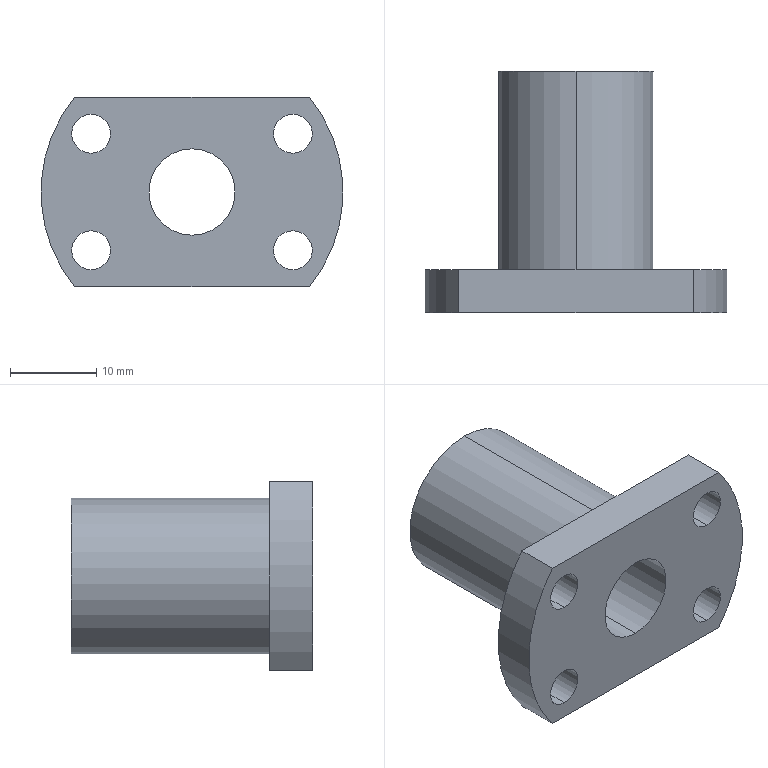Part | NX | features BREP 1 | 1 solid | 19 faces | box 35 x 28 x 22 mm | volume 6914 mm3 | cylinder 14 | plane 5 | commonest cylinder face diameters 4.5 x8 10 x2 18 x2 35 x2
STEP:
#1=CARTESIAN_POINT('',(-11.691,5.,-4.5));
#2=VERTEX_POINT('',#1);
#3=CARTESIAN_POINT('',(-11.691,0.,-4.5));
#4=VERTEX_POINT('',#3);
#5=CARTESIAN_POINT('',(-11.691,0.,-4.5));
#6=DIRECTION('',(0.,-1.,0.));
#7=VECTOR('',#6,1000.);
#8=LINE('',#5,#7);
#9=EDGE_CURVE('',#2,#4,#8,.T.);
#10=ORIENTED_EDGE('',*,*,#9,.F.);
#11=CARTESIAN_POINT('',(-11.691,5.,-9.));
#12=VERTEX_POINT('',#11);
#13=CARTESIAN_POINT('',(-11.691,5.,-6.75));
#14=DIRECTION('',(0.,-1.,0.));
#15=DIRECTION('',(0.,0.,-1.));
#16=AXIS2_PLACEMENT_3D('',#13,#14,#15);
#17=CIRCLE('',#16,2.25);
#18=EDGE_CURVE('',#12,#2,#17,.T.);
#19=ORIENTED_EDGE('',*,*,#18,.F.);
#20=CARTESIAN_POINT('',(-11.691,0.,-9.));
#21=VERTEX_POINT('',#20);
#22=CARTESIAN_POINT('',(-11.691,0.,-9.));
#23=DIRECTION('',(0.,-1.,0.));
#24=VECTOR('',#23,1000.);
#25=LINE('',#22,#24);
#26=EDGE_CURVE('',#12,#21,#25,.T.);
#27=ORIENTED_EDGE('',*,*,#26,.T.);
#28=CARTESIAN_POINT('',(-11.691,0.,-6.75));
#29=DIRECTION('',(0.,-1.,0.));
#30=DIRECTION('',(0.,0.,-1.));
#31=AXIS2_PLACEMENT_3D('',#28,#29,#30);
#32=CIRCLE('',#31,2.25);
#33=EDGE_CURVE('',#21,#4,#32,.T.);
#34=ORIENTED_EDGE('',*,*,#33,.T.);
#35=EDGE_LOOP('',(#10,#19,#27,#34));
#36=FACE_BOUND('',#35,.T.);
#37=CARTESIAN_POINT('',(-11.691,0.,-6.75));
#38=DIRECTION('',(0.,-1.,0.));
#39=DIRECTION('',(0.,0.,-1.));
#40=AXIS2_PLACEMENT_3D('',#37,#38,#39);
#41=CYLINDRICAL_SURFACE('',#40,2.25);
#42=ADVANCED_FACE('',(#36),#41,.F.);
#43=CARTESIAN_POINT('',(-11.691,5.,9.));
#44=VERTEX_POINT('',#43);
#45=CARTESIAN_POINT('',(-11.691,0.,9.));
#46=VERTEX_POINT('',#45);
#47=CARTESIAN_POINT('',(-11.691,0.,9.));
#48=DIRECTION('',(0.,-1.,0.));
#49=VECTOR('',#48,1000.);
#50=LINE('',#47,#49);
#51=EDGE_CURVE('',#44,#46,#50,.T.);
#52=ORIENTED_EDGE('',*,*,#51,.F.);
#53=CARTESIAN_POINT('',(-11.691,5.,4.5));
#54=VERTEX_POINT('',#53);
#55=CARTESIAN_POINT('',(-11.691,5.,6.75));
#56=DIRECTION('',(0.,-1.,0.));
#57=DIRECTION('',(0.,0.,-1.));
#58=AXIS2_PLACEMENT_3D('',#55,#56,#57);
#59=CIRCLE('',#58,2.25);
#60=EDGE_CURVE('',#54,#44,#59,.T.);
#61=ORIENTED_EDGE('',*,*,#60,.F.);
#62=CARTESIAN_POINT('',(-11.691,0.,4.5));
#63=VERTEX_POINT('',#62);
#64=CARTESIAN_POINT('',(-11.691,0.,4.5));
#65=DIRECTION('',(0.,-1.,0.));
#66=VECTOR('',#65,1000.);
#67=LINE('',#64,#66);
#68=EDGE_CURVE('',#54,#63,#67,.T.);
#69=ORIENTED_EDGE('',*,*,#68,.T.);
#70=CARTESIAN_POINT('',(-11.691,0.,6.75));
#71=DIRECTION('',(0.,-1.,0.));
#72=DIRECTION('',(0.,0.,-1.));
#73=AXIS2_PLACEMENT_3D('',#70,#71,#72);
#74=CIRCLE('',#73,2.25);
#75=EDGE_CURVE('',#63,#46,#74,.T.);
#76=ORIENTED_EDGE('',*,*,#75,.T.);
#77=EDGE_LOOP('',(#52,#61,#69,#76));
#78=FACE_BOUND('',#77,.T.);
#79=CARTESIAN_POINT('',(-11.691,0.,6.75));
#80=DIRECTION('',(0.,-1.,0.));
#81=DIRECTION('',(0.,0.,-1.));
#82=AXIS2_PLACEMENT_3D('',#79,#80,#81);
#83=CYLINDRICAL_SURFACE('',#82,2.25);
#84=ADVANCED_FACE('',(#78),#83,.F.);
#85=CARTESIAN_POINT('',(11.691,5.,-4.5));
#86=VERTEX_POINT('',#85);
#87=CARTESIAN_POINT('',(11.691,0.,-4.5));
#88=VERTEX_POINT('',#87);
#89=CARTESIAN_POINT('',(11.691,0.,-4.5));
#90=DIRECTION('',(0.,-1.,0.));
#91=VECTOR('',#90,1000.);
#92=LINE('',#89,#91);
#93=EDGE_CURVE('',#86,#88,#92,.T.);
#94=ORIENTED_EDGE('',*,*,#93,.F.);
#95=CARTESIAN_POINT('',(11.691,5.,-9.));
#96=VERTEX_POINT('',#95);
#97=CARTESIAN_POINT('',(11.691,5.,-6.75));
#98=DIRECTION('',(0.,-1.,0.));
#99=DIRECTION('',(0.,0.,-1.));
#100=AXIS2_PLACEMENT_3D('',#97,#98,#99);
#101=CIRCLE('',#100,2.25);
#102=EDGE_CURVE('',#96,#86,#101,.T.);
#103=ORIENTED_EDGE('',*,*,#102,.F.);
#104=CARTESIAN_POINT('',(11.691,0.,-9.));
#105=VERTEX_POINT('',#104);
#106=CARTESIAN_POINT('',(11.691,0.,-9.));
#107=DIRECTION('',(0.,-1.,0.));
#108=VECTOR('',#107,1000.);
#109=LINE('',#106,#108);
#110=EDGE_CURVE('',#96,#105,#109,.T.);
#111=ORIENTED_EDGE('',*,*,#110,.T.);
#112=CARTESIAN_POINT('',(11.691,0.,-6.75));
#113=DIRECTION('',(0.,-1.,0.));
#114=DIRECTION('',(0.,0.,-1.));
#115=AXIS2_PLACEMENT_3D('',#112,#113,#114);
#116=CIRCLE('',#115,2.25);
#117=EDGE_CURVE('',#105,#88,#116,.T.);
#118=ORIENTED_EDGE('',*,*,#117,.T.);
#119=EDGE_LOOP('',(#94,#103,#111,#118));
#120=FACE_BOUND('',#119,.T.);
#121=CARTESIAN_POINT('',(11.691,0.,-6.75));
#122=DIRECTION('',(0.,-1.,0.));
#123=DIRECTION('',(0.,0.,-1.));
#124=AXIS2_PLACEMENT_3D('',#121,#122,#123);
#125=CYLINDRICAL_SURFACE('',#124,2.25);
#126=ADVANCED_FACE('',(#120),#125,.F.);
#127=CARTESIAN_POINT('',(11.691,5.,9.));
#128=VERTEX_POINT('',#127);
#129=CARTESIAN_POINT('',(11.691,0.,9.));
#130=VERTEX_POINT('',#129);
#131=CARTESIAN_POINT('',(11.691,0.,9.));
#132=DIRECTION('',(0.,-1.,0.));
#133=VECTOR('',#132,1000.);
#134=LINE('',#131,#133);
#135=EDGE_CURVE('',#128,#130,#134,.T.);
#136=ORIENTED_EDGE('',*,*,#135,.F.);
#137=CARTESIAN_POINT('',(11.691,5.,4.5));
#138=VERTEX_POINT('',#137);
#139=CARTESIAN_POINT('',(11.691,5.,6.75));
#140=DIRECTION('',(0.,-1.,0.));
#141=DIRECTION('',(0.,0.,-1.));
#142=AXIS2_PLACEMENT_3D('',#139,#140,#141);
#143=CIRCLE('',#142,2.25);
#144=EDGE_CURVE('',#138,#128,#143,.T.);
#145=ORIENTED_EDGE('',*,*,#144,.F.);
#146=CARTESIAN_POINT('',(11.691,0.,4.5));
#147=VERTEX_POINT('',#146);
#148=CARTESIAN_POINT('',(11.691,0.,4.5));
#149=DIRECTION('',(0.,-1.,0.));
#150=VECTOR('',#149,1000.);
#151=LINE('',#148,#150);
#152=EDGE_CURVE('',#138,#147,#151,.T.);
#153=ORIENTED_EDGE('',*,*,#152,.T.);
#154=CARTESIAN_POINT('',(11.691,0.,6.75));
#155=DIRECTION('',(0.,-1.,0.));
#156=DIRECTION('',(0.,0.,-1.));
#157=AXIS2_PLACEMENT_3D('',#154,#155,#156);
#158=CIRCLE('',#157,2.25);
#159=EDGE_CURVE('',#147,#130,#158,.T.);
#160=ORIENTED_EDGE('',*,*,#159,.T.);
#161=EDGE_LOOP('',(#136,#145,#153,#160));
#162=FACE_BOUND('',#161,.T.);
#163=CARTESIAN_POINT('',(11.691,0.,6.75));
#164=DIRECTION('',(0.,-1.,0.));
#165=DIRECTION('',(0.,0.,-1.));
#166=AXIS2_PLACEMENT_3D('',#163,#164,#165);
#167=CYLINDRICAL_SURFACE('',#166,2.25);
#168=ADVANCED_FACE('',(#162),#167,.F.);
#169=CARTESIAN_POINT('',(-13.611,0.,11.));
#170=VERTEX_POINT('',#169);
#171=CARTESIAN_POINT('',(-13.611,5.,11.));
#172=VERTEX_POINT('',#171);
#173=CARTESIAN_POINT('',(-13.611,0.,11.));
#174=DIRECTION('',(0.,1.,0.));
#175=VECTOR('',#174,1000.);
#176=LINE('',#173,#175);
#177=EDGE_CURVE('',#170,#172,#176,.T.);
#178=ORIENTED_EDGE('',*,*,#177,.F.);
#179=CARTESIAN_POINT('',(13.611,0.,11.));
#180=VERTEX_POINT('',#179);
#181=CARTESIAN_POINT('',(13.611,0.,11.));
#182=DIRECTION('',(1.,0.,0.));
#183=VECTOR('',#182,1000.);
#184=LINE('',#181,#183);
#185=EDGE_CURVE('',#170,#180,#184,.T.);
#186=ORIENTED_EDGE('',*,*,#185,.T.);
#187=CARTESIAN_POINT('',(13.611,5.,11.));
#188=VERTEX_POINT('',#187);
#189=CARTESIAN_POINT('',(13.611,0.,11.));
#190=DIRECTION('',(0.,-1.,0.));
#191=VECTOR('',#190,1000.);
#192=LINE('',#189,#191);
#193=EDGE_CURVE('',#188,#180,#192,.T.);
#194=ORIENTED_EDGE('',*,*,#193,.F.);
#195=CARTESIAN_POINT('',(-9.,5.,11.));
#196=DIRECTION('',(1.,0.,0.));
#197=VECTOR('',#196,1000.);
#198=LINE('',#195,#197);
#199=EDGE_CURVE('',#172,#188,#198,.T.);
#200=ORIENTED_EDGE('',*,*,#199,.F.);
#201=EDGE_LOOP('',(#178,#186,#194,#200));
#202=FACE_BOUND('',#201,.T.);
#203=CARTESIAN_POINT('',(13.611,10.,11.));
#204=DIRECTION('',(0.,0.,-1.));
#205=DIRECTION('',(-1.,0.,0.));
#206=AXIS2_PLACEMENT_3D('',#203,#204,#205);
#207=PLANE('',#206);
#208=ADVANCED_FACE('',(#202),#207,.F.);
#209=CARTESIAN_POINT('',(13.611,0.,-11.));
#210=VERTEX_POINT('',#209);
#211=CARTESIAN_POINT('',(13.611,5.,-11.));
#212=VERTEX_POINT('',#211);
#213=CARTESIAN_POINT('',(13.611,0.,-11.));
#214=DIRECTION('',(0.,1.,0.));
#215=VECTOR('',#214,1000.);
#216=LINE('',#213,#215);
#217=EDGE_CURVE('',#210,#212,#216,.T.);
#218=ORIENTED_EDGE('',*,*,#217,.F.);
#219=CARTESIAN_POINT('',(-13.611,0.,-11.));
#220=VERTEX_POINT('',#219);
#221=CARTESIAN_POINT('',(13.611,0.,-11.));
#222=DIRECTION('',(-1.,0.,0.));
#223=VECTOR('',#222,1000.);
#224=LINE('',#221,#223);
#225=EDGE_CURVE('',#210,#220,#224,.T.);
#226=ORIENTED_EDGE('',*,*,#225,.T.);
#227=CARTESIAN_POINT('',(-13.611,5.,-11.));
#228=VERTEX_POINT('',#227);
#229=CARTESIAN_POINT('',(-13.611,0.,-11.));
#230=DIRECTION('',(0.,-1.,0.));
#231=VECTOR('',#230,1000.);
#232=LINE('',#229,#231);
#233=EDGE_CURVE('',#228,#220,#232,.T.);
#234=ORIENTED_EDGE('',*,*,#233,.F.);
#235=CARTESIAN_POINT('',(-9.,5.,-11.));
#236=DIRECTION('',(-1.,0.,0.));
#237=VECTOR('',#236,1000.);
#238=LINE('',#235,#237);
#239=EDGE_CURVE('',#212,#228,#238,.T.);
#240=ORIENTED_EDGE('',*,*,#239,.F.);
#241=EDGE_LOOP('',(#218,#226,#234,#240));
#242=FACE_BOUND('',#241,.T.);
#243=CARTESIAN_POINT('',(13.611,10.,-11.));
#244=DIRECTION('',(0.,0.,1.));
#245=DIRECTION('',(1.,0.,0.));
#246=AXIS2_PLACEMENT_3D('',#243,#244,#245);
#247=PLANE('',#246);
#248=ADVANCED_FACE('',(#242),#247,.F.);
#249=CARTESIAN_POINT('',(0.,0.,0.));
#250=DIRECTION('',(0.,-1.,0.));
#251=DIRECTION('',(0.,0.,-1.));
#252=AXIS2_PLACEMENT_3D('',#249,#250,#251);
#253=CIRCLE('',#252,17.5);
#254=EDGE_CURVE('',#170,#220,#253,.T.);
#255=ORIENTED_EDGE('',*,*,#254,.F.);
#256=ORIENTED_EDGE('',*,*,#177,.T.);
#257=CARTESIAN_POINT('',(0.,5.,0.));
#258=DIRECTION('',(0.,-1.,0.));
#259=DIRECTION('',(0.,0.,-1.));
#260=AXIS2_PLACEMENT_3D('',#257,#258,#259);
#261=CIRCLE('',#260,17.5);
#262=EDGE_CURVE('',#172,#228,#261,.T.);
#263=ORIENTED_EDGE('',*,*,#262,.T.);
#264=ORIENTED_EDGE('',*,*,#233,.T.);
#265=EDGE_LOOP('',(#255,#256,#263,#264));
#266=FACE_BOUND('',#265,.T.);
#267=CARTESIAN_POINT('',(0.,0.,0.));
#268=DIRECTION('',(0.,-1.,0.));
#269=DIRECTION('',(0.,0.,-1.));
#270=AXIS2_PLACEMENT_3D('',#267,#268,#269);
#271=CYLINDRICAL_SURFACE('',#270,17.5);
#272=ADVANCED_FACE('',(#266),#271,.T.);
#273=CARTESIAN_POINT('',(0.,5.,-9.));
#274=VERTEX_POINT('',#273);
#275=CARTESIAN_POINT('',(0.,5.,9.));
#276=VERTEX_POINT('',#275);
#277=CARTESIAN_POINT('',(0.,5.,0.));
#278=DIRECTION('',(0.,-1.,0.));
#279=DIRECTION('',(0.,0.,-1.));
#280=AXIS2_PLACEMENT_3D('',#277,#278,#279);
#281=CIRCLE('',#280,9.);
#282=EDGE_CURVE('',#274,#276,#281,.T.);
#283=ORIENTED_EDGE('',*,*,#282,.T.);
#284=CARTESIAN_POINT('',(0.,5.,0.));
#285=DIRECTION('',(0.,-1.,0.));
#286=DIRECTION('',(0.,0.,-1.));
#287=AXIS2_PLACEMENT_3D('',#284,#285,#286);
#288=CIRCLE('',#287,9.);
#289=EDGE_CURVE('',#276,#274,#288,.T.);
#290=ORIENTED_EDGE('',*,*,#289,.T.);
#291=EDGE_LOOP('',(#283,#290));
#292=FACE_BOUND('',#291,.T.);
#293=ORIENTED_EDGE('',*,*,#262,.F.);
#294=ORIENTED_EDGE('',*,*,#199,.T.);
#295=CARTESIAN_POINT('',(0.,5.,0.));
#296=DIRECTION('',(0.,-1.,0.));
#297=DIRECTION('',(0.,0.,-1.));
#298=AXIS2_PLACEMENT_3D('',#295,#296,#297);
#299=CIRCLE('',#298,17.5);
#300=EDGE_CURVE('',#212,#188,#299,.T.);
#301=ORIENTED_EDGE('',*,*,#300,.F.);
#302=ORIENTED_EDGE('',*,*,#239,.T.);
#303=EDGE_LOOP('',(#293,#294,#301,#302));
#304=FACE_BOUND('',#303,.T.);
#305=ORIENTED_EDGE('',*,*,#144,.T.);
#306=CARTESIAN_POINT('',(11.691,5.,6.75));
#307=DIRECTION('',(0.,-1.,0.));
#308=DIRECTION('',(0.,0.,-1.));
#309=AXIS2_PLACEMENT_3D('',#306,#307,#308);
#310=CIRCLE('',#309,2.25);
#311=EDGE_CURVE('',#128,#138,#310,.T.);
#312=ORIENTED_EDGE('',*,*,#311,.T.);
#313=EDGE_LOOP('',(#305,#312));
#314=FACE_BOUND('',#313,.T.);
#315=ORIENTED_EDGE('',*,*,#102,.T.);
#316=CARTESIAN_POINT('',(11.691,5.,-6.75));
#317=DIRECTION('',(0.,-1.,0.));
#318=DIRECTION('',(0.,0.,-1.));
#319=AXIS2_PLACEMENT_3D('',#316,#317,#318);
#320=CIRCLE('',#319,2.25);
#321=EDGE_CURVE('',#86,#96,#320,.T.);
#322=ORIENTED_EDGE('',*,*,#321,.T.);
#323=EDGE_LOOP('',(#315,#322));
#324=FACE_BOUND('',#323,.T.);
#325=ORIENTED_EDGE('',*,*,#60,.T.);
#326=CARTESIAN_POINT('',(-11.691,5.,6.75));
#327=DIRECTION('',(0.,-1.,0.));
#328=DIRECTION('',(0.,0.,-1.));
#329=AXIS2_PLACEMENT_3D('',#326,#327,#328);
#330=CIRCLE('',#329,2.25);
#331=EDGE_CURVE('',#44,#54,#330,.T.);
#332=ORIENTED_EDGE('',*,*,#331,.T.);
#333=EDGE_LOOP('',(#325,#332));
#334=FACE_BOUND('',#333,.T.);
#335=ORIENTED_EDGE('',*,*,#18,.T.);
#336=CARTESIAN_POINT('',(-11.691,5.,-6.75));
#337=DIRECTION('',(0.,-1.,0.));
#338=DIRECTION('',(0.,0.,-1.));
#339=AXIS2_PLACEMENT_3D('',#336,#337,#338);
#340=CIRCLE('',#339,2.25);
#341=EDGE_CURVE('',#2,#12,#340,.T.);
#342=ORIENTED_EDGE('',*,*,#341,.T.);
#343=EDGE_LOOP('',(#335,#342));
#344=FACE_BOUND('',#343,.T.);
#345=CARTESIAN_POINT('',(-9.,5.,0.));
#346=DIRECTION('',(0.,-1.,0.));
#347=DIRECTION('',(0.,0.,-1.));
#348=AXIS2_PLACEMENT_3D('',#345,#346,#347);
#349=PLANE('',#348);
#350=ADVANCED_FACE('',(#292,#304,#314,#324,#334,#344),#349,.F.);
#351=CARTESIAN_POINT('',(0.,28.,9.));
#352=VERTEX_POINT('',#351);
#353=CARTESIAN_POINT('',(0.,0.,9.));
#354=DIRECTION('',(0.,-1.,0.));
#355=VECTOR('',#354,1000.);
#356=LINE('',#353,#355);
#357=EDGE_CURVE('',#352,#276,#356,.T.);
#358=ORIENTED_EDGE('',*,*,#357,.F.);
#359=CARTESIAN_POINT('',(0.,28.,-9.));
#360=VERTEX_POINT('',#359);
#361=CARTESIAN_POINT('',(0.,28.,0.));
#362=DIRECTION('',(0.,-1.,0.));
#363=DIRECTION('',(0.,0.,-1.));
#364=AXIS2_PLACEMENT_3D('',#361,#362,#363);
#365=CIRCLE('',#364,9.);
#366=EDGE_CURVE('',#352,#360,#365,.T.);
#367=ORIENTED_EDGE('',*,*,#366,.T.);
#368=CARTESIAN_POINT('',(0.,0.,-9.));
#369=DIRECTION('',(0.,-1.,0.));
#370=VECTOR('',#369,1000.);
#371=LINE('',#368,#370);
#372=EDGE_CURVE('',#360,#274,#371,.T.);
#373=ORIENTED_EDGE('',*,*,#372,.T.);
#374=ORIENTED_EDGE('',*,*,#289,.F.);
#375=EDGE_LOOP('',(#358,#367,#373,#374));
#376=FACE_BOUND('',#375,.T.);
#377=CARTESIAN_POINT('',(0.,0.,0.));
#378=DIRECTION('',(0.,-1.,0.));
#379=DIRECTION('',(0.,0.,-1.));
#380=AXIS2_PLACEMENT_3D('',#377,#378,#379);
#381=CYLINDRICAL_SURFACE('',#380,9.);
#382=ADVANCED_FACE('',(#376),#381,.T.);
#383=CARTESIAN_POINT('',(0.,28.,-5.));
#384=VERTEX_POINT('',#383);
#385=CARTESIAN_POINT('',(0.,28.,5.));
#386=VERTEX_POINT('',#385);
#387=CARTESIAN_POINT('',(0.,28.,0.));
#388=DIRECTION('',(0.,-1.,0.));
#389=DIRECTION('',(0.,0.,-1.));
#390=AXIS2_PLACEMENT_3D('',#387,#388,#389);
#391=CIRCLE('',#390,5.);
#392=EDGE_CURVE('',#384,#386,#391,.T.);
#393=ORIENTED_EDGE('',*,*,#392,.T.);
#394=CARTESIAN_POINT('',(0.,28.,0.));
#395=DIRECTION('',(0.,-1.,0.));
#396=DIRECTION('',(0.,0.,-1.));
#397=AXIS2_PLACEMENT_3D('',#394,#395,#396);
#398=CIRCLE('',#397,5.);
#399=EDGE_CURVE('',#386,#384,#398,.T.);
#400=ORIENTED_EDGE('',*,*,#399,.T.);
#401=EDGE_LOOP('',(#393,#400));
#402=FACE_BOUND('',#401,.T.);
#403=CARTESIAN_POINT('',(0.,28.,0.));
#404=DIRECTION('',(0.,-1.,0.));
#405=DIRECTION('',(0.,0.,-1.));
#406=AXIS2_PLACEMENT_3D('',#403,#404,#405);
#407=CIRCLE('',#406,9.);
#408=EDGE_CURVE('',#360,#352,#407,.T.);
#409=ORIENTED_EDGE('',*,*,#408,.F.);
#410=ORIENTED_EDGE('',*,*,#366,.F.);
#411=EDGE_LOOP('',(#409,#410));
#412=FACE_BOUND('',#411,.T.);
#413=CARTESIAN_POINT('',(-5.,28.,0.));
#414=DIRECTION('',(0.,-1.,0.));
#415=DIRECTION('',(0.,0.,-1.));
#416=AXIS2_PLACEMENT_3D('',#413,#414,#415);
#417=PLANE('',#416);
#418=ADVANCED_FACE('',(#402,#412),#417,.F.);
#419=CARTESIAN_POINT('',(0.,0.,5.));
#420=VERTEX_POINT('',#419);
#421=CARTESIAN_POINT('',(0.,0.,5.));
#422=DIRECTION('',(0.,-1.,0.));
#423=VECTOR('',#422,1000.);
#424=LINE('',#421,#423);
#425=EDGE_CURVE('',#386,#420,#424,.T.);
#426=ORIENTED_EDGE('',*,*,#425,.F.);
#427=ORIENTED_EDGE('',*,*,#392,.F.);
#428=CARTESIAN_POINT('',(0.,0.,-5.));
#429=VERTEX_POINT('',#428);
#430=CARTESIAN_POINT('',(0.,0.,-5.));
#431=DIRECTION('',(0.,-1.,0.));
#432=VECTOR('',#431,1000.);
#433=LINE('',#430,#432);
#434=EDGE_CURVE('',#384,#429,#433,.T.);
#435=ORIENTED_EDGE('',*,*,#434,.T.);
#436=CARTESIAN_POINT('',(0.,0.,0.));
#437=DIRECTION('',(0.,-1.,0.));
#438=DIRECTION('',(0.,0.,-1.));
#439=AXIS2_PLACEMENT_3D('',#436,#437,#438);
#440=CIRCLE('',#439,5.);
#441=EDGE_CURVE('',#429,#420,#440,.T.);
#442=ORIENTED_EDGE('',*,*,#441,.T.);
#443=EDGE_LOOP('',(#426,#427,#435,#442));
#444=FACE_BOUND('',#443,.T.);
#445=CARTESIAN_POINT('',(0.,0.,0.));
#446=DIRECTION('',(0.,-1.,0.));
#447=DIRECTION('',(0.,0.,-1.));
#448=AXIS2_PLACEMENT_3D('',#445,#446,#447);
#449=CYLINDRICAL_SURFACE('',#448,5.);
#450=ADVANCED_FACE('',(#444),#449,.F.);
#451=ORIENTED_EDGE('',*,*,#300,.T.);
#452=ORIENTED_EDGE('',*,*,#193,.T.);
#453=CARTESIAN_POINT('',(0.,0.,0.));
#454=DIRECTION('',(0.,-1.,0.));
#455=DIRECTION('',(0.,0.,-1.));
#456=AXIS2_PLACEMENT_3D('',#453,#454,#455);
#457=CIRCLE('',#456,17.5);
#458=EDGE_CURVE('',#210,#180,#457,.T.);
#459=ORIENTED_EDGE('',*,*,#458,.F.);
#460=ORIENTED_EDGE('',*,*,#217,.T.);
#461=EDGE_LOOP('',(#451,#452,#459,#460));
#462=FACE_BOUND('',#461,.T.);
#463=CARTESIAN_POINT('',(0.,0.,0.));
#464=DIRECTION('',(0.,-1.,0.));
#465=DIRECTION('',(0.,0.,-1.));
#466=AXIS2_PLACEMENT_3D('',#463,#464,#465);
#467=CYLINDRICAL_SURFACE('',#466,17.5);
#468=ADVANCED_FACE('',(#462),#467,.T.);
#469=ORIENTED_EDGE('',*,*,#33,.F.);
#470=CARTESIAN_POINT('',(-11.691,0.,-6.75));
#471=DIRECTION('',(0.,-1.,0.));
#472=DIRECTION('',(0.,0.,-1.));
#473=AXIS2_PLACEMENT_3D('',#470,#471,#472);
#474=CIRCLE('',#473,2.25);
#475=EDGE_CURVE('',#4,#21,#474,.T.);
#476=ORIENTED_EDGE('',*,*,#475,.F.);
#477=EDGE_LOOP('',(#469,#476));
#478=FACE_BOUND('',#477,.T.);
#479=ORIENTED_EDGE('',*,*,#75,.F.);
#480=CARTESIAN_POINT('',(-11.691,0.,6.75));
#481=DIRECTION('',(0.,-1.,0.));
#482=DIRECTION('',(0.,0.,-1.));
#483=AXIS2_PLACEMENT_3D('',#480,#481,#482);
#484=CIRCLE('',#483,2.25);
#485=EDGE_CURVE('',#46,#63,#484,.T.);
#486=ORIENTED_EDGE('',*,*,#485,.F.);
#487=EDGE_LOOP('',(#479,#486));
#488=FACE_BOUND('',#487,.T.);
#489=ORIENTED_EDGE('',*,*,#117,.F.);
#490=CARTESIAN_POINT('',(11.691,0.,-6.75));
#491=DIRECTION('',(0.,-1.,0.));
#492=DIRECTION('',(0.,0.,-1.));
#493=AXIS2_PLACEMENT_3D('',#490,#491,#492);
#494=CIRCLE('',#493,2.25);
#495=EDGE_CURVE('',#88,#105,#494,.T.);
#496=ORIENTED_EDGE('',*,*,#495,.F.);
#497=EDGE_LOOP('',(#489,#496));
#498=FACE_BOUND('',#497,.T.);
#499=ORIENTED_EDGE('',*,*,#159,.F.);
#500=CARTESIAN_POINT('',(11.691,0.,6.75));
#501=DIRECTION('',(0.,-1.,0.));
#502=DIRECTION('',(0.,0.,-1.));
#503=AXIS2_PLACEMENT_3D('',#500,#501,#502);
#504=CIRCLE('',#503,2.25);
#505=EDGE_CURVE('',#130,#147,#504,.T.);
#506=ORIENTED_EDGE('',*,*,#505,.F.);
#507=EDGE_LOOP('',(#499,#506));
#508=FACE_BOUND('',#507,.T.);
#509=ORIENTED_EDGE('',*,*,#458,.T.);
#510=ORIENTED_EDGE('',*,*,#185,.F.);
#511=ORIENTED_EDGE('',*,*,#254,.T.);
#512=ORIENTED_EDGE('',*,*,#225,.F.);
#513=EDGE_LOOP('',(#509,#510,#511,#512));
#514=FACE_BOUND('',#513,.T.);
#515=ORIENTED_EDGE('',*,*,#441,.F.);
#516=CARTESIAN_POINT('',(0.,0.,0.));
#517=DIRECTION('',(0.,-1.,0.));
#518=DIRECTION('',(0.,0.,-1.));
#519=AXIS2_PLACEMENT_3D('',#516,#517,#518);
#520=CIRCLE('',#519,5.);
#521=EDGE_CURVE('',#420,#429,#520,.T.);
#522=ORIENTED_EDGE('',*,*,#521,.F.);
#523=EDGE_LOOP('',(#515,#522));
#524=FACE_BOUND('',#523,.T.);
#525=CARTESIAN_POINT('',(-17.5,0.,0.));
#526=DIRECTION('',(0.,1.,0.));
#527=DIRECTION('',(0.,0.,1.));
#528=AXIS2_PLACEMENT_3D('',#525,#526,#527);
#529=PLANE('',#528);
#530=ADVANCED_FACE('',(#478,#488,#498,#508,#514,#524),#529,.F.);
#531=ORIENTED_EDGE('',*,*,#399,.F.);
#532=ORIENTED_EDGE('',*,*,#425,.T.);
#533=ORIENTED_EDGE('',*,*,#521,.T.);
#534=ORIENTED_EDGE('',*,*,#434,.F.);
#535=EDGE_LOOP('',(#531,#532,#533,#534));
#536=FACE_BOUND('',#535,.T.);
#537=CARTESIAN_POINT('',(0.,0.,0.));
#538=DIRECTION('',(0.,-1.,0.));
#539=DIRECTION('',(0.,0.,-1.));
#540=AXIS2_PLACEMENT_3D('',#537,#538,#539);
#541=CYLINDRICAL_SURFACE('',#540,5.);
#542=ADVANCED_FACE('',(#536),#541,.F.);
#543=ORIENTED_EDGE('',*,*,#408,.T.);
#544=ORIENTED_EDGE('',*,*,#357,.T.);
#545=ORIENTED_EDGE('',*,*,#282,.F.);
#546=ORIENTED_EDGE('',*,*,#372,.F.);
#547=EDGE_LOOP('',(#543,#544,#545,#546));
#548=FACE_BOUND('',#547,.T.);
#549=CARTESIAN_POINT('',(0.,0.,0.));
#550=DIRECTION('',(0.,-1.,0.));
#551=DIRECTION('',(0.,0.,-1.));
#552=AXIS2_PLACEMENT_3D('',#549,#550,#551);
#553=CYLINDRICAL_SURFACE('',#552,9.);
#554=ADVANCED_FACE('',(#548),#553,.T.);
#555=ORIENTED_EDGE('',*,*,#311,.F.);
#556=ORIENTED_EDGE('',*,*,#135,.T.);
#557=ORIENTED_EDGE('',*,*,#505,.T.);
#558=ORIENTED_EDGE('',*,*,#152,.F.);
#559=EDGE_LOOP('',(#555,#556,#557,#558));
#560=FACE_BOUND('',#559,.T.);
#561=CARTESIAN_POINT('',(11.691,0.,6.75));
#562=DIRECTION('',(0.,-1.,0.));
#563=DIRECTION('',(0.,0.,-1.));
#564=AXIS2_PLACEMENT_3D('',#561,#562,#563);
#565=CYLINDRICAL_SURFACE('',#564,2.25);
#566=ADVANCED_FACE('',(#560),#565,.F.);
#567=ORIENTED_EDGE('',*,*,#321,.F.);
#568=ORIENTED_EDGE('',*,*,#93,.T.);
#569=ORIENTED_EDGE('',*,*,#495,.T.);
#570=ORIENTED_EDGE('',*,*,#110,.F.);
#571=EDGE_LOOP('',(#567,#568,#569,#570));
#572=FACE_BOUND('',#571,.T.);
#573=CARTESIAN_POINT('',(11.691,0.,-6.75));
#574=DIRECTION('',(0.,-1.,0.));
#575=DIRECTION('',(0.,0.,-1.));
#576=AXIS2_PLACEMENT_3D('',#573,#574,#575);
#577=CYLINDRICAL_SURFACE('',#576,2.25);
#578=ADVANCED_FACE('',(#572),#577,.F.);
#579=ORIENTED_EDGE('',*,*,#331,.F.);
#580=ORIENTED_EDGE('',*,*,#51,.T.);
#581=ORIENTED_EDGE('',*,*,#485,.T.);
#582=ORIENTED_EDGE('',*,*,#68,.F.);
#583=EDGE_LOOP('',(#579,#580,#581,#582));
#584=FACE_BOUND('',#583,.T.);
#585=CARTESIAN_POINT('',(-11.691,0.,6.75));
#586=DIRECTION('',(0.,-1.,0.));
#587=DIRECTION('',(0.,0.,-1.));
#588=AXIS2_PLACEMENT_3D('',#585,#586,#587);
#589=CYLINDRICAL_SURFACE('',#588,2.25);
#590=ADVANCED_FACE('',(#584),#589,.F.);
#591=ORIENTED_EDGE('',*,*,#341,.F.);
#592=ORIENTED_EDGE('',*,*,#9,.T.);
#593=ORIENTED_EDGE('',*,*,#475,.T.);
#594=ORIENTED_EDGE('',*,*,#26,.F.);
#595=EDGE_LOOP('',(#591,#592,#593,#594));
#596=FACE_BOUND('',#595,.T.);
#597=CARTESIAN_POINT('',(-11.691,0.,-6.75));
#598=DIRECTION('',(0.,-1.,0.));
#599=DIRECTION('',(0.,0.,-1.));
#600=AXIS2_PLACEMENT_3D('',#597,#598,#599);
#601=CYLINDRICAL_SURFACE('',#600,2.25);
#602=ADVANCED_FACE('',(#596),#601,.F.);
#603=CLOSED_SHELL('',(#42,#84,#126,#168,#208,#248,#272,#350,#382,#418,#450,#468,#530,#542,#554,#566,#578,#590,#602));
#604=MANIFOLD_SOLID_BREP('',#603);
#605=(LENGTH_UNIT()NAMED_UNIT(*)SI_UNIT(.MILLI.,.METRE.));
#606=UNCERTAINTY_MEASURE_WITH_UNIT(LENGTH_MEASURE(0.00001),#605,'','');
#607=(NAMED_UNIT(*)PLANE_ANGLE_UNIT()SI_UNIT($,.RADIAN.));
#608=(NAMED_UNIT(*)SI_UNIT($,.STERADIAN.)SOLID_ANGLE_UNIT());
#609=(GEOMETRIC_REPRESENTATION_CONTEXT(3)GLOBAL_UNCERTAINTY_ASSIGNED_CONTEXT((#606))GLOBAL_UNIT_ASSIGNED_CONTEXT((#605,#607,#608))REPRESENTATION_CONTEXT('',''));
#610=ADVANCED_BREP_SHAPE_REPRESENTATION('',(#604),#609);